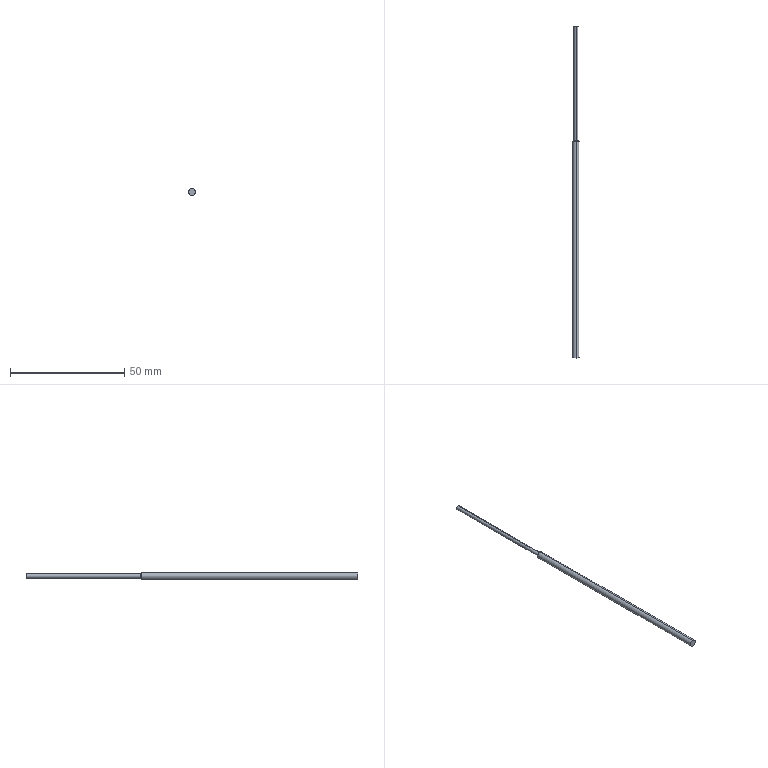Part | SolidWorks | features ICE 4, Chamfer 2, MoveFace 2, Extrusion 1 | 1 solid | 8 faces | box 3 x 145 x 3 mm | volume 797.28 mm3 | cylinder 4 | cone 2 | plane 2 | commonest cylinder face diameters 1.8 x2 3 x2
STEP:
#1=CARTESIAN_POINT('',(0.,20.,-0.9));
#2=VERTEX_POINT('',#1);
#3=CARTESIAN_POINT('',(0.,20.,0.9));
#4=VERTEX_POINT('',#3);
#5=CARTESIAN_POINT('',(0.,20.,0.));
#6=DIRECTION('',(0.,-1.,0.));
#7=DIRECTION('',(0.,0.,-1.));
#8=AXIS2_PLACEMENT_3D('',#5,#6,#7);
#9=CIRCLE('',#8,0.9);
#10=EDGE_CURVE('',#2,#4,#9,.T.);
#11=ORIENTED_EDGE('',*,*,#10,.T.);
#12=CARTESIAN_POINT('',(0.,19.4,1.5));
#13=VERTEX_POINT('',#12);
#14=CARTESIAN_POINT('',(0.,19.4,1.5));
#15=DIRECTION('',(0.,-0.7071,0.7071));
#16=VECTOR('',#15,1000.);
#17=LINE('',#14,#16);
#18=EDGE_CURVE('',#4,#13,#17,.T.);
#19=ORIENTED_EDGE('',*,*,#18,.T.);
#20=CARTESIAN_POINT('',(0.,19.4,-1.5));
#21=VERTEX_POINT('',#20);
#22=CARTESIAN_POINT('',(0.,19.4,0.));
#23=DIRECTION('',(0.,-1.,0.));
#24=DIRECTION('',(0.,0.,-1.));
#25=AXIS2_PLACEMENT_3D('',#22,#23,#24);
#26=CIRCLE('',#25,1.5);
#27=EDGE_CURVE('',#21,#13,#26,.T.);
#28=ORIENTED_EDGE('',*,*,#27,.F.);
#29=CARTESIAN_POINT('',(0.,19.4,-1.5));
#30=DIRECTION('',(0.,-0.7071,-0.7071));
#31=VECTOR('',#30,1000.);
#32=LINE('',#29,#31);
#33=EDGE_CURVE('',#2,#21,#32,.T.);
#34=ORIENTED_EDGE('',*,*,#33,.F.);
#35=EDGE_LOOP('',(#11,#19,#28,#34));
#36=FACE_OUTER_BOUND('',#35,.T.);
#37=CARTESIAN_POINT('',(0.,19.4,0.));
#38=DIRECTION('',(0.,-1.,0.));
#39=DIRECTION('',(0.,0.,-1.));
#40=AXIS2_PLACEMENT_3D('',#37,#38,#39);
#41=CONICAL_SURFACE('',#40,1.5,0.7854);
#42=ADVANCED_FACE('',(#36),#41,.T.);
#43=CARTESIAN_POINT('',(0.,70.,0.9));
#44=VERTEX_POINT('',#43);
#45=CARTESIAN_POINT('',(0.,70.,-0.9));
#46=VERTEX_POINT('',#45);
#47=CARTESIAN_POINT('',(0.,70.,0.));
#48=DIRECTION('',(0.,1.,0.));
#49=DIRECTION('',(0.,0.,1.));
#50=AXIS2_PLACEMENT_3D('',#47,#48,#49);
#51=CIRCLE('',#50,0.9);
#52=EDGE_CURVE('',#44,#46,#51,.T.);
#53=ORIENTED_EDGE('',*,*,#52,.F.);
#54=CARTESIAN_POINT('',(0.,65.,0.9));
#55=DIRECTION('',(0.,-1.,0.));
#56=VECTOR('',#55,1000.);
#57=LINE('',#54,#56);
#58=EDGE_CURVE('',#44,#4,#57,.T.);
#59=ORIENTED_EDGE('',*,*,#58,.T.);
#60=ORIENTED_EDGE('',*,*,#10,.F.);
#61=CARTESIAN_POINT('',(0.,65.,-0.9));
#62=DIRECTION('',(0.,-1.,0.));
#63=VECTOR('',#62,1000.);
#64=LINE('',#61,#63);
#65=EDGE_CURVE('',#46,#2,#64,.T.);
#66=ORIENTED_EDGE('',*,*,#65,.F.);
#67=EDGE_LOOP('',(#53,#59,#60,#66));
#68=FACE_OUTER_BOUND('',#67,.T.);
#69=CARTESIAN_POINT('',(0.,65.,0.));
#70=DIRECTION('',(0.,-1.,0.));
#71=DIRECTION('',(0.,0.,-1.));
#72=AXIS2_PLACEMENT_3D('',#69,#70,#71);
#73=CYLINDRICAL_SURFACE('',#72,0.9);
#74=ADVANCED_FACE('',(#68),#73,.T.);
#75=ORIENTED_EDGE('',*,*,#27,.T.);
#76=CARTESIAN_POINT('',(0.,-75.,1.5));
#77=VERTEX_POINT('',#76);
#78=CARTESIAN_POINT('',(0.,20.,1.5));
#79=DIRECTION('',(0.,-1.,0.));
#80=VECTOR('',#79,1000.);
#81=LINE('',#78,#80);
#82=EDGE_CURVE('',#13,#77,#81,.T.);
#83=ORIENTED_EDGE('',*,*,#82,.T.);
#84=CARTESIAN_POINT('',(0.,-75.,-1.5));
#85=VERTEX_POINT('',#84);
#86=CARTESIAN_POINT('',(0.,-75.,0.));
#87=DIRECTION('',(0.,1.,0.));
#88=DIRECTION('',(0.,0.,1.));
#89=AXIS2_PLACEMENT_3D('',#86,#87,#88);
#90=CIRCLE('',#89,1.5);
#91=EDGE_CURVE('',#77,#85,#90,.T.);
#92=ORIENTED_EDGE('',*,*,#91,.T.);
#93=CARTESIAN_POINT('',(0.,20.,-1.5));
#94=DIRECTION('',(0.,-1.,0.));
#95=VECTOR('',#94,1000.);
#96=LINE('',#93,#95);
#97=EDGE_CURVE('',#21,#85,#96,.T.);
#98=ORIENTED_EDGE('',*,*,#97,.F.);
#99=EDGE_LOOP('',(#75,#83,#92,#98));
#100=FACE_OUTER_BOUND('',#99,.T.);
#101=CARTESIAN_POINT('',(0.,20.,0.));
#102=DIRECTION('',(0.,-1.,0.));
#103=DIRECTION('',(0.,0.,-1.));
#104=AXIS2_PLACEMENT_3D('',#101,#102,#103);
#105=CYLINDRICAL_SURFACE('',#104,1.5);
#106=ADVANCED_FACE('',(#100),#105,.T.);
#107=ORIENTED_EDGE('',*,*,#82,.F.);
#108=CARTESIAN_POINT('',(0.,19.4,0.));
#109=DIRECTION('',(0.,-1.,0.));
#110=DIRECTION('',(0.,0.,-1.));
#111=AXIS2_PLACEMENT_3D('',#108,#109,#110);
#112=CIRCLE('',#111,1.5);
#113=EDGE_CURVE('',#13,#21,#112,.T.);
#114=ORIENTED_EDGE('',*,*,#113,.T.);
#115=ORIENTED_EDGE('',*,*,#97,.T.);
#116=CARTESIAN_POINT('',(0.,-75.,0.));
#117=DIRECTION('',(0.,1.,0.));
#118=DIRECTION('',(0.,0.,1.));
#119=AXIS2_PLACEMENT_3D('',#116,#117,#118);
#120=CIRCLE('',#119,1.5);
#121=EDGE_CURVE('',#85,#77,#120,.T.);
#122=ORIENTED_EDGE('',*,*,#121,.T.);
#123=EDGE_LOOP('',(#107,#114,#115,#122));
#124=FACE_OUTER_BOUND('',#123,.T.);
#125=CARTESIAN_POINT('',(0.,20.,0.));
#126=DIRECTION('',(0.,-1.,0.));
#127=DIRECTION('',(0.,0.,-1.));
#128=AXIS2_PLACEMENT_3D('',#125,#126,#127);
#129=CYLINDRICAL_SURFACE('',#128,1.5);
#130=ADVANCED_FACE('',(#124),#129,.T.);
#131=CARTESIAN_POINT('',(0.,70.,0.));
#132=DIRECTION('',(0.,1.,0.));
#133=DIRECTION('',(0.,0.,1.));
#134=AXIS2_PLACEMENT_3D('',#131,#132,#133);
#135=CIRCLE('',#134,0.9);
#136=EDGE_CURVE('',#46,#44,#135,.T.);
#137=ORIENTED_EDGE('',*,*,#136,.T.);
#138=ORIENTED_EDGE('',*,*,#52,.T.);
#139=EDGE_LOOP('',(#137,#138));
#140=FACE_OUTER_BOUND('',#139,.T.);
#141=CARTESIAN_POINT('',(0.,70.,0.));
#142=DIRECTION('',(0.,1.,0.));
#143=DIRECTION('',(0.,0.,1.));
#144=AXIS2_PLACEMENT_3D('',#141,#142,#143);
#145=PLANE('',#144);
#146=ADVANCED_FACE('',(#140),#145,.T.);
#147=ORIENTED_EDGE('',*,*,#58,.F.);
#148=ORIENTED_EDGE('',*,*,#136,.F.);
#149=ORIENTED_EDGE('',*,*,#65,.T.);
#150=CARTESIAN_POINT('',(0.,20.,0.));
#151=DIRECTION('',(0.,-1.,0.));
#152=DIRECTION('',(0.,0.,-1.));
#153=AXIS2_PLACEMENT_3D('',#150,#151,#152);
#154=CIRCLE('',#153,0.9);
#155=EDGE_CURVE('',#4,#2,#154,.T.);
#156=ORIENTED_EDGE('',*,*,#155,.F.);
#157=EDGE_LOOP('',(#147,#148,#149,#156));
#158=FACE_OUTER_BOUND('',#157,.T.);
#159=CARTESIAN_POINT('',(0.,65.,0.));
#160=DIRECTION('',(0.,-1.,0.));
#161=DIRECTION('',(0.,0.,-1.));
#162=AXIS2_PLACEMENT_3D('',#159,#160,#161);
#163=CYLINDRICAL_SURFACE('',#162,0.9);
#164=ADVANCED_FACE('',(#158),#163,.T.);
#165=ORIENTED_EDGE('',*,*,#18,.F.);
#166=ORIENTED_EDGE('',*,*,#155,.T.);
#167=ORIENTED_EDGE('',*,*,#33,.T.);
#168=ORIENTED_EDGE('',*,*,#113,.F.);
#169=EDGE_LOOP('',(#165,#166,#167,#168));
#170=FACE_OUTER_BOUND('',#169,.T.);
#171=CARTESIAN_POINT('',(0.,19.4,0.));
#172=DIRECTION('',(0.,-1.,0.));
#173=DIRECTION('',(0.,0.,-1.));
#174=AXIS2_PLACEMENT_3D('',#171,#172,#173);
#175=CONICAL_SURFACE('',#174,1.5,0.7854);
#176=ADVANCED_FACE('',(#170),#175,.T.);
#177=ORIENTED_EDGE('',*,*,#121,.F.);
#178=ORIENTED_EDGE('',*,*,#91,.F.);
#179=EDGE_LOOP('',(#177,#178));
#180=FACE_OUTER_BOUND('',#179,.T.);
#181=CARTESIAN_POINT('',(0.,-75.,0.));
#182=DIRECTION('',(0.,1.,0.));
#183=DIRECTION('',(0.,0.,1.));
#184=AXIS2_PLACEMENT_3D('',#181,#182,#183);
#185=PLANE('',#184);
#186=ADVANCED_FACE('',(#180),#185,.F.);
#187=CLOSED_SHELL('',(#42,#74,#106,#130,#146,#164,#176,#186));
#188=MANIFOLD_SOLID_BREP('',#187);
#189=CARTESIAN_POINT('',(0.,0.,0.));
#190=DIRECTION('',(0.,0.,1.));
#191=DIRECTION('',(1.,0.,0.));
#192=AXIS2_PLACEMENT_3D('',#189,#190,#191);
#193=(LENGTH_UNIT()NAMED_UNIT(*)SI_UNIT(.MILLI.,.METRE.));
#194=UNCERTAINTY_MEASURE_WITH_UNIT(LENGTH_MEASURE(0.00001),#193,'','');
#195=(NAMED_UNIT(*)PLANE_ANGLE_UNIT()SI_UNIT($,.RADIAN.));
#196=(NAMED_UNIT(*)SI_UNIT($,.STERADIAN.)SOLID_ANGLE_UNIT());
#197=(GEOMETRIC_REPRESENTATION_CONTEXT(3)GLOBAL_UNCERTAINTY_ASSIGNED_CONTEXT((#194))GLOBAL_UNIT_ASSIGNED_CONTEXT((#193,#195,#196))REPRESENTATION_CONTEXT('',''));
#198=ADVANCED_BREP_SHAPE_REPRESENTATION('',(#188,#192),#197);